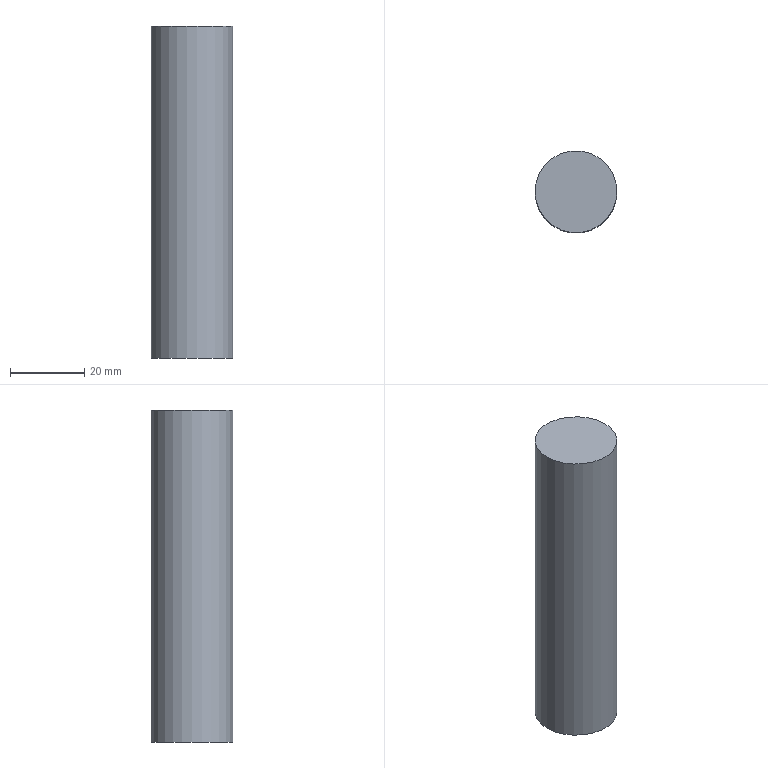Part | STEP file | solid 106 | 1 solid | 3 faces | box 22 x 22 x 89.177 mm | volume 33899 mm3 | plane 2 | cylinder 1 | commonest cylinder face diameters 22 x1